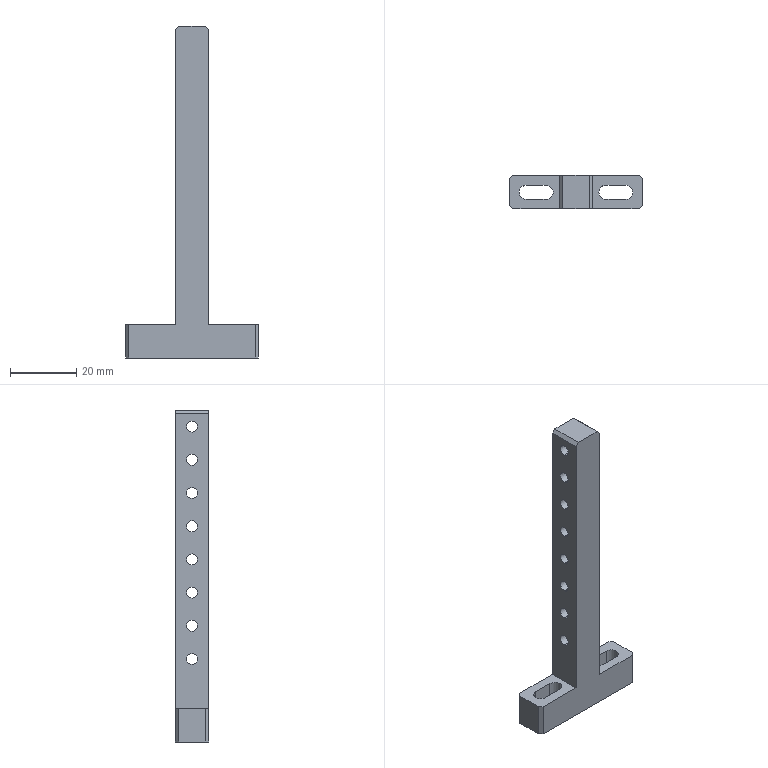Part | SolidWorks | features ICE 3, Chamfer 1, Extrusion 1, HoleWzd 1 | 1 solid | 42 faces | box 40 x 10 x 100 mm | volume 11505 mm3 | cylinder 22 | plane 20 | commonest cylinder face diameters 3.3 x16 4.2 x6
STEP:
#1=CARTESIAN_POINT('',(-5.,0.,26.65));
#2=VERTEX_POINT('',#1);
#3=CARTESIAN_POINT('',(-5.,0.,23.35));
#4=VERTEX_POINT('',#3);
#5=CARTESIAN_POINT('',(-5.,0.,25.));
#6=DIRECTION('',(1.,0.,0.));
#7=DIRECTION('',(0.,0.,-1.));
#8=AXIS2_PLACEMENT_3D('',#5,#6,#7);
#9=CIRCLE('',#8,1.65);
#10=EDGE_CURVE('',#2,#4,#9,.T.);
#11=ORIENTED_EDGE('',*,*,#10,.F.);
#12=CARTESIAN_POINT('',(5.,0.,26.65));
#13=VERTEX_POINT('',#12);
#14=CARTESIAN_POINT('',(5.,0.,26.65));
#15=DIRECTION('',(1.,0.,0.));
#16=VECTOR('',#15,1000.);
#17=LINE('',#14,#16);
#18=EDGE_CURVE('',#2,#13,#17,.T.);
#19=ORIENTED_EDGE('',*,*,#18,.T.);
#20=CARTESIAN_POINT('',(5.,0.,23.35));
#21=VERTEX_POINT('',#20);
#22=CARTESIAN_POINT('',(5.,0.,25.));
#23=DIRECTION('',(1.,0.,0.));
#24=DIRECTION('',(0.,0.,-1.));
#25=AXIS2_PLACEMENT_3D('',#22,#23,#24);
#26=CIRCLE('',#25,1.65);
#27=EDGE_CURVE('',#13,#21,#26,.T.);
#28=ORIENTED_EDGE('',*,*,#27,.T.);
#29=CARTESIAN_POINT('',(5.,0.,23.35));
#30=DIRECTION('',(1.,0.,0.));
#31=VECTOR('',#30,1000.);
#32=LINE('',#29,#31);
#33=EDGE_CURVE('',#4,#21,#32,.T.);
#34=ORIENTED_EDGE('',*,*,#33,.F.);
#35=EDGE_LOOP('',(#11,#19,#28,#34));
#36=FACE_OUTER_BOUND('',#35,.T.);
#37=CARTESIAN_POINT('',(5.,0.,25.));
#38=DIRECTION('',(1.,0.,0.));
#39=DIRECTION('',(0.,0.,-1.));
#40=AXIS2_PLACEMENT_3D('',#37,#38,#39);
#41=CYLINDRICAL_SURFACE('',#40,1.65);
#42=ADVANCED_FACE('',(#36),#41,.F.);
#43=CARTESIAN_POINT('',(-5.,0.,36.65));
#44=VERTEX_POINT('',#43);
#45=CARTESIAN_POINT('',(-5.,0.,33.35));
#46=VERTEX_POINT('',#45);
#47=CARTESIAN_POINT('',(-5.,0.,35.));
#48=DIRECTION('',(1.,0.,0.));
#49=DIRECTION('',(0.,0.,-1.));
#50=AXIS2_PLACEMENT_3D('',#47,#48,#49);
#51=CIRCLE('',#50,1.65);
#52=EDGE_CURVE('',#44,#46,#51,.T.);
#53=ORIENTED_EDGE('',*,*,#52,.F.);
#54=CARTESIAN_POINT('',(5.,0.,36.65));
#55=VERTEX_POINT('',#54);
#56=CARTESIAN_POINT('',(5.,0.,36.65));
#57=DIRECTION('',(1.,0.,0.));
#58=VECTOR('',#57,1000.);
#59=LINE('',#56,#58);
#60=EDGE_CURVE('',#44,#55,#59,.T.);
#61=ORIENTED_EDGE('',*,*,#60,.T.);
#62=CARTESIAN_POINT('',(5.,0.,33.35));
#63=VERTEX_POINT('',#62);
#64=CARTESIAN_POINT('',(5.,0.,35.));
#65=DIRECTION('',(1.,0.,0.));
#66=DIRECTION('',(0.,0.,-1.));
#67=AXIS2_PLACEMENT_3D('',#64,#65,#66);
#68=CIRCLE('',#67,1.65);
#69=EDGE_CURVE('',#55,#63,#68,.T.);
#70=ORIENTED_EDGE('',*,*,#69,.T.);
#71=CARTESIAN_POINT('',(5.,0.,33.35));
#72=DIRECTION('',(1.,0.,0.));
#73=VECTOR('',#72,1000.);
#74=LINE('',#71,#73);
#75=EDGE_CURVE('',#46,#63,#74,.T.);
#76=ORIENTED_EDGE('',*,*,#75,.F.);
#77=EDGE_LOOP('',(#53,#61,#70,#76));
#78=FACE_OUTER_BOUND('',#77,.T.);
#79=CARTESIAN_POINT('',(5.,0.,35.));
#80=DIRECTION('',(1.,0.,0.));
#81=DIRECTION('',(0.,0.,-1.));
#82=AXIS2_PLACEMENT_3D('',#79,#80,#81);
#83=CYLINDRICAL_SURFACE('',#82,1.65);
#84=ADVANCED_FACE('',(#78),#83,.F.);
#85=CARTESIAN_POINT('',(-5.,0.,46.65));
#86=VERTEX_POINT('',#85);
#87=CARTESIAN_POINT('',(-5.,0.,43.35));
#88=VERTEX_POINT('',#87);
#89=CARTESIAN_POINT('',(-5.,0.,45.));
#90=DIRECTION('',(1.,0.,0.));
#91=DIRECTION('',(0.,0.,-1.));
#92=AXIS2_PLACEMENT_3D('',#89,#90,#91);
#93=CIRCLE('',#92,1.65);
#94=EDGE_CURVE('',#86,#88,#93,.T.);
#95=ORIENTED_EDGE('',*,*,#94,.F.);
#96=CARTESIAN_POINT('',(5.,0.,46.65));
#97=VERTEX_POINT('',#96);
#98=CARTESIAN_POINT('',(5.,0.,46.65));
#99=DIRECTION('',(1.,0.,0.));
#100=VECTOR('',#99,1000.);
#101=LINE('',#98,#100);
#102=EDGE_CURVE('',#86,#97,#101,.T.);
#103=ORIENTED_EDGE('',*,*,#102,.T.);
#104=CARTESIAN_POINT('',(5.,0.,43.35));
#105=VERTEX_POINT('',#104);
#106=CARTESIAN_POINT('',(5.,0.,45.));
#107=DIRECTION('',(1.,0.,0.));
#108=DIRECTION('',(0.,0.,-1.));
#109=AXIS2_PLACEMENT_3D('',#106,#107,#108);
#110=CIRCLE('',#109,1.65);
#111=EDGE_CURVE('',#97,#105,#110,.T.);
#112=ORIENTED_EDGE('',*,*,#111,.T.);
#113=CARTESIAN_POINT('',(5.,0.,43.35));
#114=DIRECTION('',(1.,0.,0.));
#115=VECTOR('',#114,1000.);
#116=LINE('',#113,#115);
#117=EDGE_CURVE('',#88,#105,#116,.T.);
#118=ORIENTED_EDGE('',*,*,#117,.F.);
#119=EDGE_LOOP('',(#95,#103,#112,#118));
#120=FACE_OUTER_BOUND('',#119,.T.);
#121=CARTESIAN_POINT('',(5.,0.,45.));
#122=DIRECTION('',(1.,0.,0.));
#123=DIRECTION('',(0.,0.,-1.));
#124=AXIS2_PLACEMENT_3D('',#121,#122,#123);
#125=CYLINDRICAL_SURFACE('',#124,1.65);
#126=ADVANCED_FACE('',(#120),#125,.F.);
#127=CARTESIAN_POINT('',(-5.,0.,56.65));
#128=VERTEX_POINT('',#127);
#129=CARTESIAN_POINT('',(-5.,0.,53.35));
#130=VERTEX_POINT('',#129);
#131=CARTESIAN_POINT('',(-5.,0.,55.));
#132=DIRECTION('',(1.,0.,0.));
#133=DIRECTION('',(0.,0.,-1.));
#134=AXIS2_PLACEMENT_3D('',#131,#132,#133);
#135=CIRCLE('',#134,1.65);
#136=EDGE_CURVE('',#128,#130,#135,.T.);
#137=ORIENTED_EDGE('',*,*,#136,.F.);
#138=CARTESIAN_POINT('',(5.,0.,56.65));
#139=VERTEX_POINT('',#138);
#140=CARTESIAN_POINT('',(5.,0.,56.65));
#141=DIRECTION('',(1.,0.,0.));
#142=VECTOR('',#141,1000.);
#143=LINE('',#140,#142);
#144=EDGE_CURVE('',#128,#139,#143,.T.);
#145=ORIENTED_EDGE('',*,*,#144,.T.);
#146=CARTESIAN_POINT('',(5.,0.,53.35));
#147=VERTEX_POINT('',#146);
#148=CARTESIAN_POINT('',(5.,0.,55.));
#149=DIRECTION('',(1.,0.,0.));
#150=DIRECTION('',(0.,0.,-1.));
#151=AXIS2_PLACEMENT_3D('',#148,#149,#150);
#152=CIRCLE('',#151,1.65);
#153=EDGE_CURVE('',#139,#147,#152,.T.);
#154=ORIENTED_EDGE('',*,*,#153,.T.);
#155=CARTESIAN_POINT('',(5.,0.,53.35));
#156=DIRECTION('',(1.,0.,0.));
#157=VECTOR('',#156,1000.);
#158=LINE('',#155,#157);
#159=EDGE_CURVE('',#130,#147,#158,.T.);
#160=ORIENTED_EDGE('',*,*,#159,.F.);
#161=EDGE_LOOP('',(#137,#145,#154,#160));
#162=FACE_OUTER_BOUND('',#161,.T.);
#163=CARTESIAN_POINT('',(5.,0.,55.));
#164=DIRECTION('',(1.,0.,0.));
#165=DIRECTION('',(0.,0.,-1.));
#166=AXIS2_PLACEMENT_3D('',#163,#164,#165);
#167=CYLINDRICAL_SURFACE('',#166,1.65);
#168=ADVANCED_FACE('',(#162),#167,.F.);
#169=CARTESIAN_POINT('',(-5.,0.,66.65));
#170=VERTEX_POINT('',#169);
#171=CARTESIAN_POINT('',(-5.,0.,63.35));
#172=VERTEX_POINT('',#171);
#173=CARTESIAN_POINT('',(-5.,0.,65.));
#174=DIRECTION('',(1.,0.,0.));
#175=DIRECTION('',(0.,0.,-1.));
#176=AXIS2_PLACEMENT_3D('',#173,#174,#175);
#177=CIRCLE('',#176,1.65);
#178=EDGE_CURVE('',#170,#172,#177,.T.);
#179=ORIENTED_EDGE('',*,*,#178,.F.);
#180=CARTESIAN_POINT('',(5.,0.,66.65));
#181=VERTEX_POINT('',#180);
#182=CARTESIAN_POINT('',(5.,0.,66.65));
#183=DIRECTION('',(1.,0.,0.));
#184=VECTOR('',#183,1000.);
#185=LINE('',#182,#184);
#186=EDGE_CURVE('',#170,#181,#185,.T.);
#187=ORIENTED_EDGE('',*,*,#186,.T.);
#188=CARTESIAN_POINT('',(5.,0.,63.35));
#189=VERTEX_POINT('',#188);
#190=CARTESIAN_POINT('',(5.,0.,65.));
#191=DIRECTION('',(1.,0.,0.));
#192=DIRECTION('',(0.,0.,-1.));
#193=AXIS2_PLACEMENT_3D('',#190,#191,#192);
#194=CIRCLE('',#193,1.65);
#195=EDGE_CURVE('',#181,#189,#194,.T.);
#196=ORIENTED_EDGE('',*,*,#195,.T.);
#197=CARTESIAN_POINT('',(5.,0.,63.35));
#198=DIRECTION('',(1.,0.,0.));
#199=VECTOR('',#198,1000.);
#200=LINE('',#197,#199);
#201=EDGE_CURVE('',#172,#189,#200,.T.);
#202=ORIENTED_EDGE('',*,*,#201,.F.);
#203=EDGE_LOOP('',(#179,#187,#196,#202));
#204=FACE_OUTER_BOUND('',#203,.T.);
#205=CARTESIAN_POINT('',(5.,0.,65.));
#206=DIRECTION('',(1.,0.,0.));
#207=DIRECTION('',(0.,0.,-1.));
#208=AXIS2_PLACEMENT_3D('',#205,#206,#207);
#209=CYLINDRICAL_SURFACE('',#208,1.65);
#210=ADVANCED_FACE('',(#204),#209,.F.);
#211=CARTESIAN_POINT('',(-5.,0.,76.65));
#212=VERTEX_POINT('',#211);
#213=CARTESIAN_POINT('',(-5.,0.,73.35));
#214=VERTEX_POINT('',#213);
#215=CARTESIAN_POINT('',(-5.,0.,75.));
#216=DIRECTION('',(1.,0.,0.));
#217=DIRECTION('',(0.,0.,-1.));
#218=AXIS2_PLACEMENT_3D('',#215,#216,#217);
#219=CIRCLE('',#218,1.65);
#220=EDGE_CURVE('',#212,#214,#219,.T.);
#221=ORIENTED_EDGE('',*,*,#220,.F.);
#222=CARTESIAN_POINT('',(5.,0.,76.65));
#223=VERTEX_POINT('',#222);
#224=CARTESIAN_POINT('',(5.,0.,76.65));
#225=DIRECTION('',(1.,0.,0.));
#226=VECTOR('',#225,1000.);
#227=LINE('',#224,#226);
#228=EDGE_CURVE('',#212,#223,#227,.T.);
#229=ORIENTED_EDGE('',*,*,#228,.T.);
#230=CARTESIAN_POINT('',(5.,0.,73.35));
#231=VERTEX_POINT('',#230);
#232=CARTESIAN_POINT('',(5.,0.,75.));
#233=DIRECTION('',(1.,0.,0.));
#234=DIRECTION('',(0.,0.,-1.));
#235=AXIS2_PLACEMENT_3D('',#232,#233,#234);
#236=CIRCLE('',#235,1.65);
#237=EDGE_CURVE('',#223,#231,#236,.T.);
#238=ORIENTED_EDGE('',*,*,#237,.T.);
#239=CARTESIAN_POINT('',(5.,0.,73.35));
#240=DIRECTION('',(1.,0.,0.));
#241=VECTOR('',#240,1000.);
#242=LINE('',#239,#241);
#243=EDGE_CURVE('',#214,#231,#242,.T.);
#244=ORIENTED_EDGE('',*,*,#243,.F.);
#245=EDGE_LOOP('',(#221,#229,#238,#244));
#246=FACE_OUTER_BOUND('',#245,.T.);
#247=CARTESIAN_POINT('',(5.,0.,75.));
#248=DIRECTION('',(1.,0.,0.));
#249=DIRECTION('',(0.,0.,-1.));
#250=AXIS2_PLACEMENT_3D('',#247,#248,#249);
#251=CYLINDRICAL_SURFACE('',#250,1.65);
#252=ADVANCED_FACE('',(#246),#251,.F.);
#253=CARTESIAN_POINT('',(-5.,0.,86.65));
#254=VERTEX_POINT('',#253);
#255=CARTESIAN_POINT('',(-5.,0.,83.35));
#256=VERTEX_POINT('',#255);
#257=CARTESIAN_POINT('',(-5.,0.,85.));
#258=DIRECTION('',(1.,0.,0.));
#259=DIRECTION('',(0.,0.,-1.));
#260=AXIS2_PLACEMENT_3D('',#257,#258,#259);
#261=CIRCLE('',#260,1.65);
#262=EDGE_CURVE('',#254,#256,#261,.T.);
#263=ORIENTED_EDGE('',*,*,#262,.F.);
#264=CARTESIAN_POINT('',(5.,0.,86.65));
#265=VERTEX_POINT('',#264);
#266=CARTESIAN_POINT('',(5.,0.,86.65));
#267=DIRECTION('',(1.,0.,0.));
#268=VECTOR('',#267,1000.);
#269=LINE('',#266,#268);
#270=EDGE_CURVE('',#254,#265,#269,.T.);
#271=ORIENTED_EDGE('',*,*,#270,.T.);
#272=CARTESIAN_POINT('',(5.,0.,83.35));
#273=VERTEX_POINT('',#272);
#274=CARTESIAN_POINT('',(5.,0.,85.));
#275=DIRECTION('',(1.,0.,0.));
#276=DIRECTION('',(0.,0.,-1.));
#277=AXIS2_PLACEMENT_3D('',#274,#275,#276);
#278=CIRCLE('',#277,1.65);
#279=EDGE_CURVE('',#265,#273,#278,.T.);
#280=ORIENTED_EDGE('',*,*,#279,.T.);
#281=CARTESIAN_POINT('',(5.,0.,83.35));
#282=DIRECTION('',(1.,0.,0.));
#283=VECTOR('',#282,1000.);
#284=LINE('',#281,#283);
#285=EDGE_CURVE('',#256,#273,#284,.T.);
#286=ORIENTED_EDGE('',*,*,#285,.F.);
#287=EDGE_LOOP('',(#263,#271,#280,#286));
#288=FACE_OUTER_BOUND('',#287,.T.);
#289=CARTESIAN_POINT('',(5.,0.,85.));
#290=DIRECTION('',(1.,0.,0.));
#291=DIRECTION('',(0.,0.,-1.));
#292=AXIS2_PLACEMENT_3D('',#289,#290,#291);
#293=CYLINDRICAL_SURFACE('',#292,1.65);
#294=ADVANCED_FACE('',(#288),#293,.F.);
#295=CARTESIAN_POINT('',(-5.,0.,96.65));
#296=VERTEX_POINT('',#295);
#297=CARTESIAN_POINT('',(-5.,0.,93.35));
#298=VERTEX_POINT('',#297);
#299=CARTESIAN_POINT('',(-5.,0.,95.));
#300=DIRECTION('',(1.,0.,0.));
#301=DIRECTION('',(0.,0.,-1.));
#302=AXIS2_PLACEMENT_3D('',#299,#300,#301);
#303=CIRCLE('',#302,1.65);
#304=EDGE_CURVE('',#296,#298,#303,.T.);
#305=ORIENTED_EDGE('',*,*,#304,.F.);
#306=CARTESIAN_POINT('',(5.,0.,96.65));
#307=VERTEX_POINT('',#306);
#308=CARTESIAN_POINT('',(5.,0.,96.65));
#309=DIRECTION('',(1.,0.,0.));
#310=VECTOR('',#309,1000.);
#311=LINE('',#308,#310);
#312=EDGE_CURVE('',#296,#307,#311,.T.);
#313=ORIENTED_EDGE('',*,*,#312,.T.);
#314=CARTESIAN_POINT('',(5.,0.,93.35));
#315=VERTEX_POINT('',#314);
#316=CARTESIAN_POINT('',(5.,0.,95.));
#317=DIRECTION('',(1.,0.,0.));
#318=DIRECTION('',(0.,0.,-1.));
#319=AXIS2_PLACEMENT_3D('',#316,#317,#318);
#320=CIRCLE('',#319,1.65);
#321=EDGE_CURVE('',#307,#315,#320,.T.);
#322=ORIENTED_EDGE('',*,*,#321,.T.);
#323=CARTESIAN_POINT('',(5.,0.,93.35));
#324=DIRECTION('',(1.,0.,0.));
#325=VECTOR('',#324,1000.);
#326=LINE('',#323,#325);
#327=EDGE_CURVE('',#298,#315,#326,.T.);
#328=ORIENTED_EDGE('',*,*,#327,.F.);
#329=EDGE_LOOP('',(#305,#313,#322,#328));
#330=FACE_OUTER_BOUND('',#329,.T.);
#331=CARTESIAN_POINT('',(5.,0.,95.));
#332=DIRECTION('',(1.,0.,0.));
#333=DIRECTION('',(0.,0.,-1.));
#334=AXIS2_PLACEMENT_3D('',#331,#332,#333);
#335=CYLINDRICAL_SURFACE('',#334,1.65);
#336=ADVANCED_FACE('',(#330),#335,.F.);
#337=CARTESIAN_POINT('',(-15.,2.1,10.));
#338=VERTEX_POINT('',#337);
#339=CARTESIAN_POINT('',(-17.1,0.,10.));
#340=VERTEX_POINT('',#339);
#341=CARTESIAN_POINT('',(-15.,0.,10.));
#342=DIRECTION('',(0.,0.,1.));
#343=DIRECTION('',(1.,0.,0.));
#344=AXIS2_PLACEMENT_3D('',#341,#342,#343);
#345=CIRCLE('',#344,2.1);
#346=EDGE_CURVE('',#338,#340,#345,.T.);
#347=ORIENTED_EDGE('',*,*,#346,.T.);
#348=CARTESIAN_POINT('',(-17.1,0.,0.));
#349=VERTEX_POINT('',#348);
#350=CARTESIAN_POINT('',(-17.1,0.,100.));
#351=DIRECTION('',(0.,0.,-1.));
#352=VECTOR('',#351,1000.);
#353=LINE('',#350,#352);
#354=EDGE_CURVE('',#340,#349,#353,.T.);
#355=ORIENTED_EDGE('',*,*,#354,.T.);
#356=CARTESIAN_POINT('',(-15.,2.1,0.));
#357=VERTEX_POINT('',#356);
#358=CARTESIAN_POINT('',(-15.,0.,0.));
#359=DIRECTION('',(0.,0.,-1.));
#360=DIRECTION('',(1.,0.,0.));
#361=AXIS2_PLACEMENT_3D('',#358,#359,#360);
#362=CIRCLE('',#361,2.1);
#363=EDGE_CURVE('',#349,#357,#362,.T.);
#364=ORIENTED_EDGE('',*,*,#363,.T.);
#365=CARTESIAN_POINT('',(-15.,2.1,100.));
#366=DIRECTION('',(0.,0.,-1.));
#367=VECTOR('',#366,1000.);
#368=LINE('',#365,#367);
#369=EDGE_CURVE('',#338,#357,#368,.T.);
#370=ORIENTED_EDGE('',*,*,#369,.F.);
#371=EDGE_LOOP('',(#347,#355,#364,#370));
#372=FACE_OUTER_BOUND('',#371,.T.);
#373=CARTESIAN_POINT('',(-15.,0.,100.));
#374=DIRECTION('',(0.,0.,-1.));
#375=DIRECTION('',(-1.,0.,0.));
#376=AXIS2_PLACEMENT_3D('',#373,#374,#375);
#377=CYLINDRICAL_SURFACE('',#376,2.1);
#378=ADVANCED_FACE('',(#372),#377,.F.);
#379=CARTESIAN_POINT('',(9.,2.1,10.));
#380=VERTEX_POINT('',#379);
#381=CARTESIAN_POINT('',(6.9,0.,10.));
#382=VERTEX_POINT('',#381);
#383=CARTESIAN_POINT('',(9.,0.,10.));
#384=DIRECTION('',(0.,0.,1.));
#385=DIRECTION('',(1.,0.,0.));
#386=AXIS2_PLACEMENT_3D('',#383,#384,#385);
#387=CIRCLE('',#386,2.1);
#388=EDGE_CURVE('',#380,#382,#387,.T.);
#389=ORIENTED_EDGE('',*,*,#388,.T.);
#390=CARTESIAN_POINT('',(6.9,0.,0.));
#391=VERTEX_POINT('',#390);
#392=CARTESIAN_POINT('',(6.9,0.,100.));
#393=DIRECTION('',(0.,0.,-1.));
#394=VECTOR('',#393,1000.);
#395=LINE('',#392,#394);
#396=EDGE_CURVE('',#382,#391,#395,.T.);
#397=ORIENTED_EDGE('',*,*,#396,.T.);
#398=CARTESIAN_POINT('',(9.,2.1,0.));
#399=VERTEX_POINT('',#398);
#400=CARTESIAN_POINT('',(9.,0.,0.));
#401=DIRECTION('',(0.,0.,-1.));
#402=DIRECTION('',(-1.,0.,0.));
#403=AXIS2_PLACEMENT_3D('',#400,#401,#402);
#404=CIRCLE('',#403,2.1);
#405=EDGE_CURVE('',#391,#399,#404,.T.);
#406=ORIENTED_EDGE('',*,*,#405,.T.);
#407=CARTESIAN_POINT('',(9.,2.1,100.));
#408=DIRECTION('',(0.,0.,-1.));
#409=VECTOR('',#408,1000.);
#410=LINE('',#407,#409);
#411=EDGE_CURVE('',#380,#399,#410,.T.);
#412=ORIENTED_EDGE('',*,*,#411,.F.);
#413=EDGE_LOOP('',(#389,#397,#406,#412));
#414=FACE_OUTER_BOUND('',#413,.T.);
#415=CARTESIAN_POINT('',(9.,0.,100.));
#416=DIRECTION('',(0.,0.,-1.));
#417=DIRECTION('',(-1.,0.,0.));
#418=AXIS2_PLACEMENT_3D('',#415,#416,#417);
#419=CYLINDRICAL_SURFACE('',#418,2.1);
#420=ADVANCED_FACE('',(#414),#419,.F.);
#421=CARTESIAN_POINT('',(15.,-2.1,10.));
#422=VERTEX_POINT('',#421);
#423=CARTESIAN_POINT('',(15.,2.1,10.));
#424=VERTEX_POINT('',#423);
#425=CARTESIAN_POINT('',(15.,0.,10.));
#426=DIRECTION('',(0.,0.,1.));
#427=DIRECTION('',(1.,0.,0.));
#428=AXIS2_PLACEMENT_3D('',#425,#426,#427);
#429=CIRCLE('',#428,2.1);
#430=EDGE_CURVE('',#422,#424,#429,.T.);
#431=ORIENTED_EDGE('',*,*,#430,.F.);
#432=CARTESIAN_POINT('',(9.,-2.1,10.));
#433=VERTEX_POINT('',#432);
#434=CARTESIAN_POINT('',(20.,-2.1,10.));
#435=DIRECTION('',(1.,0.,0.));
#436=VECTOR('',#435,1000.);
#437=LINE('',#434,#436);
#438=EDGE_CURVE('',#433,#422,#437,.T.);
#439=ORIENTED_EDGE('',*,*,#438,.F.);
#440=CARTESIAN_POINT('',(9.,0.,10.));
#441=DIRECTION('',(0.,0.,1.));
#442=DIRECTION('',(1.,0.,0.));
#443=AXIS2_PLACEMENT_3D('',#440,#441,#442);
#444=CIRCLE('',#443,2.1);
#445=EDGE_CURVE('',#382,#433,#444,.T.);
#446=ORIENTED_EDGE('',*,*,#445,.F.);
#447=ORIENTED_EDGE('',*,*,#388,.F.);
#448=CARTESIAN_POINT('',(20.,2.1,10.));
#449=DIRECTION('',(-1.,0.,0.));
#450=VECTOR('',#449,1000.);
#451=LINE('',#448,#450);
#452=EDGE_CURVE('',#424,#380,#451,.T.);
#453=ORIENTED_EDGE('',*,*,#452,.F.);
#454=EDGE_LOOP('',(#431,#439,#446,#447,#453));
#455=FACE_BOUND('',#454,.T.);
#456=CARTESIAN_POINT('',(20.,-4.,10.));
#457=VERTEX_POINT('',#456);
#458=CARTESIAN_POINT('',(20.,4.,10.));
#459=VERTEX_POINT('',#458);
#460=CARTESIAN_POINT('',(20.,5.,10.));
#461=DIRECTION('',(0.,1.,0.));
#462=VECTOR('',#461,1000.);
#463=LINE('',#460,#462);
#464=EDGE_CURVE('',#457,#459,#463,.T.);
#465=ORIENTED_EDGE('',*,*,#464,.T.);
#466=CARTESIAN_POINT('',(19.,5.,10.));
#467=VERTEX_POINT('',#466);
#468=CARTESIAN_POINT('',(24.5,-0.5,10.));
#469=DIRECTION('',(-0.7071,0.7071,0.));
#470=VECTOR('',#469,1000.);
#471=LINE('',#468,#470);
#472=EDGE_CURVE('',#459,#467,#471,.T.);
#473=ORIENTED_EDGE('',*,*,#472,.T.);
#474=CARTESIAN_POINT('',(5.,5.,10.));
#475=VERTEX_POINT('',#474);
#476=CARTESIAN_POINT('',(-20.,5.,10.));
#477=DIRECTION('',(-1.,0.,0.));
#478=VECTOR('',#477,1000.);
#479=LINE('',#476,#478);
#480=EDGE_CURVE('',#467,#475,#479,.T.);
#481=ORIENTED_EDGE('',*,*,#480,.T.);
#482=CARTESIAN_POINT('',(5.,-5.,10.));
#483=VERTEX_POINT('',#482);
#484=CARTESIAN_POINT('',(5.,-5.,10.));
#485=DIRECTION('',(0.,1.,0.));
#486=VECTOR('',#485,1000.);
#487=LINE('',#484,#486);
#488=EDGE_CURVE('',#483,#475,#487,.T.);
#489=ORIENTED_EDGE('',*,*,#488,.F.);
#490=CARTESIAN_POINT('',(19.,-5.,10.));
#491=VERTEX_POINT('',#490);
#492=CARTESIAN_POINT('',(-20.,-5.,10.));
#493=DIRECTION('',(1.,0.,0.));
#494=VECTOR('',#493,1000.);
#495=LINE('',#492,#494);
#496=EDGE_CURVE('',#483,#491,#495,.T.);
#497=ORIENTED_EDGE('',*,*,#496,.T.);
#498=CARTESIAN_POINT('',(19.5,-4.5,10.));
#499=DIRECTION('',(0.7071,0.7071,0.));
#500=VECTOR('',#499,1000.);
#501=LINE('',#498,#500);
#502=EDGE_CURVE('',#491,#457,#501,.T.);
#503=ORIENTED_EDGE('',*,*,#502,.T.);
#504=EDGE_LOOP('',(#465,#473,#481,#489,#497,#503));
#505=FACE_OUTER_BOUND('',#504,.T.);
#506=CARTESIAN_POINT('',(20.,-5.,10.));
#507=DIRECTION('',(0.,0.,1.));
#508=DIRECTION('',(1.,0.,0.));
#509=AXIS2_PLACEMENT_3D('',#506,#507,#508);
#510=PLANE('',#509);
#511=ADVANCED_FACE('',(#455,#505),#510,.T.);
#512=CARTESIAN_POINT('',(20.,-4.,0.));
#513=VERTEX_POINT('',#512);
#514=CARTESIAN_POINT('',(20.,4.,0.));
#515=VERTEX_POINT('',#514);
#516=CARTESIAN_POINT('',(20.,5.,0.));
#517=DIRECTION('',(0.,1.,0.));
#518=VECTOR('',#517,1000.);
#519=LINE('',#516,#518);
#520=EDGE_CURVE('',#513,#515,#519,.T.);
#521=ORIENTED_EDGE('',*,*,#520,.T.);
#522=CARTESIAN_POINT('',(20.,4.,10.));
#523=DIRECTION('',(0.,0.,1.));
#524=VECTOR('',#523,1000.);
#525=LINE('',#522,#524);
#526=EDGE_CURVE('',#515,#459,#525,.T.);
#527=ORIENTED_EDGE('',*,*,#526,.T.);
#528=ORIENTED_EDGE('',*,*,#464,.F.);
#529=CARTESIAN_POINT('',(20.,-4.,10.));
#530=DIRECTION('',(0.,0.,-1.));
#531=VECTOR('',#530,1000.);
#532=LINE('',#529,#531);
#533=EDGE_CURVE('',#457,#513,#532,.T.);
#534=ORIENTED_EDGE('',*,*,#533,.T.);
#535=EDGE_LOOP('',(#521,#527,#528,#534));
#536=FACE_OUTER_BOUND('',#535,.T.);
#537=CARTESIAN_POINT('',(20.,5.,10.));
#538=DIRECTION('',(-1.,0.,0.));
#539=DIRECTION('',(0.,-1.,0.));
#540=AXIS2_PLACEMENT_3D('',#537,#538,#539);
#541=PLANE('',#540);
#542=ADVANCED_FACE('',(#536),#541,.F.);
#543=ORIENTED_EDGE('',*,*,#480,.F.);
#544=CARTESIAN_POINT('',(19.,5.,0.));
#545=VERTEX_POINT('',#544);
#546=CARTESIAN_POINT('',(19.,5.,10.));
#547=DIRECTION('',(0.,0.,-1.));
#548=VECTOR('',#547,1000.);
#549=LINE('',#546,#548);
#550=EDGE_CURVE('',#467,#545,#549,.T.);
#551=ORIENTED_EDGE('',*,*,#550,.T.);
#552=CARTESIAN_POINT('',(-19.,5.,0.));
#553=VERTEX_POINT('',#552);
#554=CARTESIAN_POINT('',(-20.,5.,0.));
#555=DIRECTION('',(-1.,0.,0.));
#556=VECTOR('',#555,1000.);
#557=LINE('',#554,#556);
#558=EDGE_CURVE('',#545,#553,#557,.T.);
#559=ORIENTED_EDGE('',*,*,#558,.T.);
#560=CARTESIAN_POINT('',(-19.,5.,10.));
#561=VERTEX_POINT('',#560);
#562=CARTESIAN_POINT('',(-19.,5.,10.));
#563=DIRECTION('',(0.,0.,1.));
#564=VECTOR('',#563,1000.);
#565=LINE('',#562,#564);
#566=EDGE_CURVE('',#553,#561,#565,.T.);
#567=ORIENTED_EDGE('',*,*,#566,.T.);
#568=CARTESIAN_POINT('',(-5.,5.,10.));
#569=VERTEX_POINT('',#568);
#570=CARTESIAN_POINT('',(-20.,5.,10.));
#571=DIRECTION('',(-1.,0.,0.));
#572=VECTOR('',#571,1000.);
#573=LINE('',#570,#572);
#574=EDGE_CURVE('',#569,#561,#573,.T.);
#575=ORIENTED_EDGE('',*,*,#574,.F.);
#576=CARTESIAN_POINT('',(-5.,5.,99.));
#577=VERTEX_POINT('',#576);
#578=CARTESIAN_POINT('',(-5.,5.,100.));
#579=DIRECTION('',(0.,0.,-1.));
#580=VECTOR('',#579,1000.);
#581=LINE('',#578,#580);
#582=EDGE_CURVE('',#577,#569,#581,.T.);
#583=ORIENTED_EDGE('',*,*,#582,.F.);
#584=CARTESIAN_POINT('',(-4.,5.,100.));
#585=VERTEX_POINT('',#584);
#586=CARTESIAN_POINT('',(-4.,5.,100.));
#587=DIRECTION('',(0.7071,0.,0.7071));
#588=VECTOR('',#587,1000.);
#589=LINE('',#586,#588);
#590=EDGE_CURVE('',#577,#585,#589,.T.);
#591=ORIENTED_EDGE('',*,*,#590,.T.);
#592=CARTESIAN_POINT('',(4.,5.,100.));
#593=VERTEX_POINT('',#592);
#594=CARTESIAN_POINT('',(-5.,5.,100.));
#595=DIRECTION('',(-1.,0.,0.));
#596=VECTOR('',#595,1000.);
#597=LINE('',#594,#596);
#598=EDGE_CURVE('',#593,#585,#597,.T.);
#599=ORIENTED_EDGE('',*,*,#598,.F.);
#600=CARTESIAN_POINT('',(5.,5.,99.));
#601=VERTEX_POINT('',#600);
#602=CARTESIAN_POINT('',(4.,5.,100.));
#603=DIRECTION('',(0.7071,0.,-0.7071));
#604=VECTOR('',#603,1000.);
#605=LINE('',#602,#604);
#606=EDGE_CURVE('',#593,#601,#605,.T.);
#607=ORIENTED_EDGE('',*,*,#606,.T.);
#608=CARTESIAN_POINT('',(5.,5.,100.));
#609=DIRECTION('',(0.,0.,-1.));
#610=VECTOR('',#609,1000.);
#611=LINE('',#608,#610);
#612=EDGE_CURVE('',#601,#475,#611,.T.);
#613=ORIENTED_EDGE('',*,*,#612,.T.);
#614=EDGE_LOOP('',(#543,#551,#559,#567,#575,#583,#591,#599,#607,#613));
#615=FACE_OUTER_BOUND('',#614,.T.);
#616=CARTESIAN_POINT('',(-20.,5.,10.));
#617=DIRECTION('',(0.,-1.,0.));
#618=DIRECTION('',(0.,0.,-1.));
#619=AXIS2_PLACEMENT_3D('',#616,#617,#618);
#620=PLANE('',#619);
#621=ADVANCED_FACE('',(#615),#620,.F.);
#622=CARTESIAN_POINT('',(-20.,4.,0.));
#623=VERTEX_POINT('',#622);
#624=CARTESIAN_POINT('',(-20.,-4.,0.));
#625=VERTEX_POINT('',#624);
#626=CARTESIAN_POINT('',(-20.,5.,0.));
#627=DIRECTION('',(0.,-1.,0.));
#628=VECTOR('',#627,1000.);
#629=LINE('',#626,#628);
#630=EDGE_CURVE('',#623,#625,#629,.T.);
#631=ORIENTED_EDGE('',*,*,#630,.T.);
#632=CARTESIAN_POINT('',(-20.,-4.,10.));
#633=VERTEX_POINT('',#632);
#634=CARTESIAN_POINT('',(-20.,-4.,10.));
#635=DIRECTION('',(0.,0.,1.));
#636=VECTOR('',#635,1000.);
#637=LINE('',#634,#636);
#638=EDGE_CURVE('',#625,#633,#637,.T.);
#639=ORIENTED_EDGE('',*,*,#638,.T.);
#640=CARTESIAN_POINT('',(-20.,4.,10.));
#641=VERTEX_POINT('',#640);
#642=CARTESIAN_POINT('',(-20.,5.,10.));
#643=DIRECTION('',(0.,-1.,0.));
#644=VECTOR('',#643,1000.);
#645=LINE('',#642,#644);
#646=EDGE_CURVE('',#641,#633,#645,.T.);
#647=ORIENTED_EDGE('',*,*,#646,.F.);
#648=CARTESIAN_POINT('',(-20.,4.,10.));
#649=DIRECTION('',(0.,0.,-1.));
#650=VECTOR('',#649,1000.);
#651=LINE('',#648,#650);
#652=EDGE_CURVE('',#641,#623,#651,.T.);
#653=ORIENTED_EDGE('',*,*,#652,.T.);
#654=EDGE_LOOP('',(#631,#639,#647,#653));
#655=FACE_OUTER_BOUND('',#654,.T.);
#656=CARTESIAN_POINT('',(-20.,5.,10.));
#657=DIRECTION('',(1.,0.,0.));
#658=DIRECTION('',(0.,0.,-1.));
#659=AXIS2_PLACEMENT_3D('',#656,#657,#658);
#660=PLANE('',#659);
#661=ADVANCED_FACE('',(#655),#660,.F.);
#662=CARTESIAN_POINT('',(-19.,-5.,0.));
#663=VERTEX_POINT('',#662);
#664=CARTESIAN_POINT('',(19.,-5.,0.));
#665=VERTEX_POINT('',#664);
#666=CARTESIAN_POINT('',(-20.,-5.,0.));
#667=DIRECTION('',(1.,0.,0.));
#668=VECTOR('',#667,1000.);
#669=LINE('',#666,#668);
#670=EDGE_CURVE('',#663,#665,#669,.T.);
#671=ORIENTED_EDGE('',*,*,#670,.T.);
#672=CARTESIAN_POINT('',(19.,-5.,10.));
#673=DIRECTION('',(0.,0.,1.));
#674=VECTOR('',#673,1000.);
#675=LINE('',#672,#674);
#676=EDGE_CURVE('',#665,#491,#675,.T.);
#677=ORIENTED_EDGE('',*,*,#676,.T.);
#678=ORIENTED_EDGE('',*,*,#496,.F.);
#679=CARTESIAN_POINT('',(5.,-5.,99.));
#680=VERTEX_POINT('',#679);
#681=CARTESIAN_POINT('',(5.,-5.,100.));
#682=DIRECTION('',(0.,0.,-1.));
#683=VECTOR('',#682,1000.);
#684=LINE('',#681,#683);
#685=EDGE_CURVE('',#680,#483,#684,.T.);
#686=ORIENTED_EDGE('',*,*,#685,.F.);
#687=CARTESIAN_POINT('',(4.,-5.,100.));
#688=VERTEX_POINT('',#687);
#689=CARTESIAN_POINT('',(4.,-5.,100.));
#690=DIRECTION('',(-0.7071,0.,0.7071));
#691=VECTOR('',#690,1000.);
#692=LINE('',#689,#691);
#693=EDGE_CURVE('',#680,#688,#692,.T.);
#694=ORIENTED_EDGE('',*,*,#693,.T.);
#695=CARTESIAN_POINT('',(-4.,-5.,100.));
#696=VERTEX_POINT('',#695);
#697=CARTESIAN_POINT('',(-5.,-5.,100.));
#698=DIRECTION('',(1.,0.,0.));
#699=VECTOR('',#698,1000.);
#700=LINE('',#697,#699);
#701=EDGE_CURVE('',#696,#688,#700,.T.);
#702=ORIENTED_EDGE('',*,*,#701,.F.);
#703=CARTESIAN_POINT('',(-5.,-5.,99.));
#704=VERTEX_POINT('',#703);
#705=CARTESIAN_POINT('',(-4.,-5.,100.));
#706=DIRECTION('',(-0.7071,0.,-0.7071));
#707=VECTOR('',#706,1000.);
#708=LINE('',#705,#707);
#709=EDGE_CURVE('',#696,#704,#708,.T.);
#710=ORIENTED_EDGE('',*,*,#709,.T.);
#711=CARTESIAN_POINT('',(-5.,-5.,10.));
#712=VERTEX_POINT('',#711);
#713=CARTESIAN_POINT('',(-5.,-5.,100.));
#714=DIRECTION('',(0.,0.,-1.));
#715=VECTOR('',#714,1000.);
#716=LINE('',#713,#715);
#717=EDGE_CURVE('',#704,#712,#716,.T.);
#718=ORIENTED_EDGE('',*,*,#717,.T.);
#719=CARTESIAN_POINT('',(-19.,-5.,10.));
#720=VERTEX_POINT('',#719);
#721=CARTESIAN_POINT('',(-20.,-5.,10.));
#722=DIRECTION('',(1.,0.,0.));
#723=VECTOR('',#722,1000.);
#724=LINE('',#721,#723);
#725=EDGE_CURVE('',#720,#712,#724,.T.);
#726=ORIENTED_EDGE('',*,*,#725,.F.);
#727=CARTESIAN_POINT('',(-19.,-5.,10.));
#728=DIRECTION('',(0.,0.,-1.));
#729=VECTOR('',#728,1000.);
#730=LINE('',#727,#729);
#731=EDGE_CURVE('',#720,#663,#730,.T.);
#732=ORIENTED_EDGE('',*,*,#731,.T.);
#733=EDGE_LOOP('',(#671,#677,#678,#686,#694,#702,#710,#718,#726,#732));
#734=FACE_OUTER_BOUND('',#733,.T.);
#735=CARTESIAN_POINT('',(-20.,-5.,10.));
#736=DIRECTION('',(0.,1.,0.));
#737=DIRECTION('',(0.,0.,1.));
#738=AXIS2_PLACEMENT_3D('',#735,#736,#737);
#739=PLANE('',#738);
#740=ADVANCED_FACE('',(#734),#739,.F.);
#741=ORIENTED_EDGE('',*,*,#346,.F.);
#742=CARTESIAN_POINT('',(-9.,2.1,10.));
#743=VERTEX_POINT('',#742);
#744=CARTESIAN_POINT('',(20.,2.1,10.));
#745=DIRECTION('',(-1.,0.,0.));
#746=VECTOR('',#745,1000.);
#747=LINE('',#744,#746);
#748=EDGE_CURVE('',#743,#338,#747,.T.);
#749=ORIENTED_EDGE('',*,*,#748,.F.);
#750=CARTESIAN_POINT('',(-9.,-2.1,10.));
#751=VERTEX_POINT('',#750);
#752=CARTESIAN_POINT('',(-9.,0.,10.));
#753=DIRECTION('',(0.,0.,1.));
#754=DIRECTION('',(1.,0.,0.));
#755=AXIS2_PLACEMENT_3D('',#752,#753,#754);
#756=CIRCLE('',#755,2.1);
#757=EDGE_CURVE('',#751,#743,#756,.T.);
#758=ORIENTED_EDGE('',*,*,#757,.F.);
#759=CARTESIAN_POINT('',(-15.,-2.1,10.));
#760=VERTEX_POINT('',#759);
#761=CARTESIAN_POINT('',(20.,-2.1,10.));
#762=DIRECTION('',(1.,0.,0.));
#763=VECTOR('',#762,1000.);
#764=LINE('',#761,#763);
#765=EDGE_CURVE('',#760,#751,#764,.T.);
#766=ORIENTED_EDGE('',*,*,#765,.F.);
#767=CARTESIAN_POINT('',(-15.,0.,10.));
#768=DIRECTION('',(0.,0.,1.));
#769=DIRECTION('',(1.,0.,0.));
#770=AXIS2_PLACEMENT_3D('',#767,#768,#769);
#771=CIRCLE('',#770,2.1);
#772=EDGE_CURVE('',#340,#760,#771,.T.);
#773=ORIENTED_EDGE('',*,*,#772,.F.);
#774=EDGE_LOOP('',(#741,#749,#758,#766,#773));
#775=FACE_BOUND('',#774,.T.);
#776=ORIENTED_EDGE('',*,*,#646,.T.);
#777=CARTESIAN_POINT('',(0.5,-24.5,10.));
#778=DIRECTION('',(0.7071,-0.7071,0.));
#779=VECTOR('',#778,1000.);
#780=LINE('',#777,#779);
#781=EDGE_CURVE('',#633,#720,#780,.T.);
#782=ORIENTED_EDGE('',*,*,#781,.T.);
#783=ORIENTED_EDGE('',*,*,#725,.T.);
#784=CARTESIAN_POINT('',(-5.,-5.,10.));
#785=DIRECTION('',(0.,-1.,0.));
#786=VECTOR('',#785,1000.);
#787=LINE('',#784,#786);
#788=EDGE_CURVE('',#569,#712,#787,.T.);
#789=ORIENTED_EDGE('',*,*,#788,.F.);
#790=ORIENTED_EDGE('',*,*,#574,.T.);
#791=CARTESIAN_POINT('',(-4.5,19.5,10.));
#792=DIRECTION('',(-0.7071,-0.7071,0.));
#793=VECTOR('',#792,1000.);
#794=LINE('',#791,#793);
#795=EDGE_CURVE('',#561,#641,#794,.T.);
#796=ORIENTED_EDGE('',*,*,#795,.T.);
#797=EDGE_LOOP('',(#776,#782,#783,#789,#790,#796));
#798=FACE_OUTER_BOUND('',#797,.T.);
#799=CARTESIAN_POINT('',(20.,-5.,10.));
#800=DIRECTION('',(0.,0.,1.));
#801=DIRECTION('',(1.,0.,0.));
#802=AXIS2_PLACEMENT_3D('',#799,#800,#801);
#803=PLANE('',#802);
#804=ADVANCED_FACE('',(#775,#798),#803,.T.);
#805=CARTESIAN_POINT('',(-9.,2.1,0.));
#806=VERTEX_POINT('',#805);
#807=CARTESIAN_POINT('',(-15.,2.1,0.));
#808=DIRECTION('',(1.,0.,0.));
#809=VECTOR('',#808,1000.);
#810=LINE('',#807,#809);
#811=EDGE_CURVE('',#357,#806,#810,.T.);
#812=ORIENTED_EDGE('',*,*,#811,.F.);
#813=ORIENTED_EDGE('',*,*,#363,.F.);
#814=CARTESIAN_POINT('',(-15.,-2.1,0.));
#815=VERTEX_POINT('',#814);
#816=CARTESIAN_POINT('',(-15.,0.,0.));
#817=DIRECTION('',(0.,0.,-1.));
#818=DIRECTION('',(1.,0.,0.));
#819=AXIS2_PLACEMENT_3D('',#816,#817,#818);
#820=CIRCLE('',#819,2.1);
#821=EDGE_CURVE('',#815,#349,#820,.T.);
#822=ORIENTED_EDGE('',*,*,#821,.F.);
#823=CARTESIAN_POINT('',(-9.,-2.1,0.));
#824=VERTEX_POINT('',#823);
#825=CARTESIAN_POINT('',(-15.,-2.1,0.));
#826=DIRECTION('',(-1.,0.,0.));
#827=VECTOR('',#826,1000.);
#828=LINE('',#825,#827);
#829=EDGE_CURVE('',#824,#815,#828,.T.);
#830=ORIENTED_EDGE('',*,*,#829,.F.);
#831=CARTESIAN_POINT('',(-9.,0.,0.));
#832=DIRECTION('',(0.,0.,-1.));
#833=DIRECTION('',(1.,0.,0.));
#834=AXIS2_PLACEMENT_3D('',#831,#832,#833);
#835=CIRCLE('',#834,2.1);
#836=EDGE_CURVE('',#806,#824,#835,.T.);
#837=ORIENTED_EDGE('',*,*,#836,.F.);
#838=EDGE_LOOP('',(#812,#813,#822,#830,#837));
#839=FACE_BOUND('',#838,.T.);
#840=CARTESIAN_POINT('',(15.,-2.1,0.));
#841=VERTEX_POINT('',#840);
#842=CARTESIAN_POINT('',(9.,-2.1,0.));
#843=VERTEX_POINT('',#842);
#844=CARTESIAN_POINT('',(15.,-2.1,0.));
#845=DIRECTION('',(-1.,0.,0.));
#846=VECTOR('',#845,1000.);
#847=LINE('',#844,#846);
#848=EDGE_CURVE('',#841,#843,#847,.T.);
#849=ORIENTED_EDGE('',*,*,#848,.F.);
#850=CARTESIAN_POINT('',(15.,2.1,0.));
#851=VERTEX_POINT('',#850);
#852=CARTESIAN_POINT('',(15.,0.,0.));
#853=DIRECTION('',(0.,0.,-1.));
#854=DIRECTION('',(-1.,0.,0.));
#855=AXIS2_PLACEMENT_3D('',#852,#853,#854);
#856=CIRCLE('',#855,2.1);
#857=EDGE_CURVE('',#851,#841,#856,.T.);
#858=ORIENTED_EDGE('',*,*,#857,.F.);
#859=CARTESIAN_POINT('',(15.,2.1,0.));
#860=DIRECTION('',(1.,0.,0.));
#861=VECTOR('',#860,1000.);
#862=LINE('',#859,#861);
#863=EDGE_CURVE('',#399,#851,#862,.T.);
#864=ORIENTED_EDGE('',*,*,#863,.F.);
#865=ORIENTED_EDGE('',*,*,#405,.F.);
#866=CARTESIAN_POINT('',(9.,0.,0.));
#867=DIRECTION('',(0.,0.,-1.));
#868=DIRECTION('',(-1.,0.,0.));
#869=AXIS2_PLACEMENT_3D('',#866,#867,#868);
#870=CIRCLE('',#869,2.1);
#871=EDGE_CURVE('',#843,#391,#870,.T.);
#872=ORIENTED_EDGE('',*,*,#871,.F.);
#873=EDGE_LOOP('',(#849,#858,#864,#865,#872));
#874=FACE_BOUND('',#873,.T.);
#875=ORIENTED_EDGE('',*,*,#558,.F.);
#876=CARTESIAN_POINT('',(19.,5.,0.));
#877=DIRECTION('',(0.7071,-0.7071,0.));
#878=VECTOR('',#877,1000.);
#879=LINE('',#876,#878);
#880=EDGE_CURVE('',#545,#515,#879,.T.);
#881=ORIENTED_EDGE('',*,*,#880,.T.);
#882=ORIENTED_EDGE('',*,*,#520,.F.);
#883=CARTESIAN_POINT('',(20.,-4.,0.));
#884=DIRECTION('',(-0.7071,-0.7071,0.));
#885=VECTOR('',#884,1000.);
#886=LINE('',#883,#885);
#887=EDGE_CURVE('',#513,#665,#886,.T.);
#888=ORIENTED_EDGE('',*,*,#887,.T.);
#889=ORIENTED_EDGE('',*,*,#670,.F.);
#890=CARTESIAN_POINT('',(-19.,-5.,0.));
#891=DIRECTION('',(-0.7071,0.7071,0.));
#892=VECTOR('',#891,1000.);
#893=LINE('',#890,#892);
#894=EDGE_CURVE('',#663,#625,#893,.T.);
#895=ORIENTED_EDGE('',*,*,#894,.T.);
#896=ORIENTED_EDGE('',*,*,#630,.F.);
#897=CARTESIAN_POINT('',(-20.,4.,0.));
#898=DIRECTION('',(0.7071,0.7071,0.));
#899=VECTOR('',#898,1000.);
#900=LINE('',#897,#899);
#901=EDGE_CURVE('',#623,#553,#900,.T.);
#902=ORIENTED_EDGE('',*,*,#901,.T.);
#903=EDGE_LOOP('',(#875,#881,#882,#888,#889,#895,#896,#902));
#904=FACE_OUTER_BOUND('',#903,.T.);
#905=CARTESIAN_POINT('',(20.,-5.,0.));
#906=DIRECTION('',(0.,0.,1.));
#907=DIRECTION('',(1.,0.,0.));
#908=AXIS2_PLACEMENT_3D('',#905,#906,#907);
#909=PLANE('',#908);
#910=ADVANCED_FACE('',(#839,#874,#904),#909,.F.);
#911=CARTESIAN_POINT('',(5.,0.,25.));
#912=DIRECTION('',(1.,0.,0.));
#913=DIRECTION('',(0.,0.,-1.));
#914=AXIS2_PLACEMENT_3D('',#911,#912,#913);
#915=CIRCLE('',#914,1.65);
#916=EDGE_CURVE('',#21,#13,#915,.T.);
#917=ORIENTED_EDGE('',*,*,#916,.F.);
#918=ORIENTED_EDGE('',*,*,#27,.F.);
#919=EDGE_LOOP('',(#917,#918));
#920=FACE_BOUND('',#919,.T.);
#921=CARTESIAN_POINT('',(5.,0.,35.));
#922=DIRECTION('',(1.,0.,0.));
#923=DIRECTION('',(0.,0.,-1.));
#924=AXIS2_PLACEMENT_3D('',#921,#922,#923);
#925=CIRCLE('',#924,1.65);
#926=EDGE_CURVE('',#63,#55,#925,.T.);
#927=ORIENTED_EDGE('',*,*,#926,.F.);
#928=ORIENTED_EDGE('',*,*,#69,.F.);
#929=EDGE_LOOP('',(#927,#928));
#930=FACE_BOUND('',#929,.T.);
#931=CARTESIAN_POINT('',(5.,0.,45.));
#932=DIRECTION('',(1.,0.,0.));
#933=DIRECTION('',(0.,0.,-1.));
#934=AXIS2_PLACEMENT_3D('',#931,#932,#933);
#935=CIRCLE('',#934,1.65);
#936=EDGE_CURVE('',#105,#97,#935,.T.);
#937=ORIENTED_EDGE('',*,*,#936,.F.);
#938=ORIENTED_EDGE('',*,*,#111,.F.);
#939=EDGE_LOOP('',(#937,#938));
#940=FACE_BOUND('',#939,.T.);
#941=CARTESIAN_POINT('',(5.,0.,55.));
#942=DIRECTION('',(1.,0.,0.));
#943=DIRECTION('',(0.,0.,-1.));
#944=AXIS2_PLACEMENT_3D('',#941,#942,#943);
#945=CIRCLE('',#944,1.65);
#946=EDGE_CURVE('',#147,#139,#945,.T.);
#947=ORIENTED_EDGE('',*,*,#946,.F.);
#948=ORIENTED_EDGE('',*,*,#153,.F.);
#949=EDGE_LOOP('',(#947,#948));
#950=FACE_BOUND('',#949,.T.);
#951=CARTESIAN_POINT('',(5.,0.,65.));
#952=DIRECTION('',(1.,0.,0.));
#953=DIRECTION('',(0.,0.,-1.));
#954=AXIS2_PLACEMENT_3D('',#951,#952,#953);
#955=CIRCLE('',#954,1.65);
#956=EDGE_CURVE('',#189,#181,#955,.T.);
#957=ORIENTED_EDGE('',*,*,#956,.F.);
#958=ORIENTED_EDGE('',*,*,#195,.F.);
#959=EDGE_LOOP('',(#957,#958));
#960=FACE_BOUND('',#959,.T.);
#961=CARTESIAN_POINT('',(5.,0.,75.));
#962=DIRECTION('',(1.,0.,0.));
#963=DIRECTION('',(0.,0.,-1.));
#964=AXIS2_PLACEMENT_3D('',#961,#962,#963);
#965=CIRCLE('',#964,1.65);
#966=EDGE_CURVE('',#231,#223,#965,.T.);
#967=ORIENTED_EDGE('',*,*,#966,.F.);
#968=ORIENTED_EDGE('',*,*,#237,.F.);
#969=EDGE_LOOP('',(#967,#968));
#970=FACE_BOUND('',#969,.T.);
#971=CARTESIAN_POINT('',(5.,0.,85.));
#972=DIRECTION('',(1.,0.,0.));
#973=DIRECTION('',(0.,0.,-1.));
#974=AXIS2_PLACEMENT_3D('',#971,#972,#973);
#975=CIRCLE('',#974,1.65);
#976=EDGE_CURVE('',#273,#265,#975,.T.);
#977=ORIENTED_EDGE('',*,*,#976,.F.);
#978=ORIENTED_EDGE('',*,*,#279,.F.);
#979=EDGE_LOOP('',(#977,#978));
#980=FACE_BOUND('',#979,.T.);
#981=CARTESIAN_POINT('',(5.,0.,95.));
#982=DIRECTION('',(1.,0.,0.));
#983=DIRECTION('',(0.,0.,-1.));
#984=AXIS2_PLACEMENT_3D('',#981,#982,#983);
#985=CIRCLE('',#984,1.65);
#986=EDGE_CURVE('',#315,#307,#985,.T.);
#987=ORIENTED_EDGE('',*,*,#986,.F.);
#988=ORIENTED_EDGE('',*,*,#321,.F.);
#989=EDGE_LOOP('',(#987,#988));
#990=FACE_BOUND('',#989,.T.);
#991=ORIENTED_EDGE('',*,*,#612,.F.);
#992=CARTESIAN_POINT('',(5.,-5.,99.));
#993=DIRECTION('',(0.,-1.,0.));
#994=VECTOR('',#993,1000.);
#995=LINE('',#992,#994);
#996=EDGE_CURVE('',#601,#680,#995,.T.);
#997=ORIENTED_EDGE('',*,*,#996,.T.);
#998=ORIENTED_EDGE('',*,*,#685,.T.);
#999=ORIENTED_EDGE('',*,*,#488,.T.);
#1000=EDGE_LOOP('',(#991,#997,#998,#999));
#1001=FACE_OUTER_BOUND('',#1000,.T.);
#1002=CARTESIAN_POINT('',(5.,-5.,100.));
#1003=DIRECTION('',(-1.,0.,0.));
#1004=DIRECTION('',(0.,0.,1.));
#1005=AXIS2_PLACEMENT_3D('',#1002,#1003,#1004);
#1006=PLANE('',#1005);
#1007=ADVANCED_FACE('',(#920,#930,#940,#950,#960,#970,#980,#990,#1001),#1006,.F.);
#1008=CARTESIAN_POINT('',(-5.,0.,25.));
#1009=DIRECTION('',(1.,0.,0.));
#1010=DIRECTION('',(0.,0.,-1.));
#1011=AXIS2_PLACEMENT_3D('',#1008,#1009,#1010);
#1012=CIRCLE('',#1011,1.65);
#1013=EDGE_CURVE('',#4,#2,#1012,.T.);
#1014=ORIENTED_EDGE('',*,*,#1013,.T.);
#1015=ORIENTED_EDGE('',*,*,#10,.T.);
#1016=EDGE_LOOP('',(#1014,#1015));
#1017=FACE_BOUND('',#1016,.T.);
#1018=CARTESIAN_POINT('',(-5.,0.,35.));
#1019=DIRECTION('',(1.,0.,0.));
#1020=DIRECTION('',(0.,0.,-1.));
#1021=AXIS2_PLACEMENT_3D('',#1018,#1019,#1020);
#1022=CIRCLE('',#1021,1.65);
#1023=EDGE_CURVE('',#46,#44,#1022,.T.);
#1024=ORIENTED_EDGE('',*,*,#1023,.T.);
#1025=ORIENTED_EDGE('',*,*,#52,.T.);
#1026=EDGE_LOOP('',(#1024,#1025));
#1027=FACE_BOUND('',#1026,.T.);
#1028=CARTESIAN_POINT('',(-5.,0.,45.));
#1029=DIRECTION('',(1.,0.,0.));
#1030=DIRECTION('',(0.,0.,-1.));
#1031=AXIS2_PLACEMENT_3D('',#1028,#1029,#1030);
#1032=CIRCLE('',#1031,1.65);
#1033=EDGE_CURVE('',#88,#86,#1032,.T.);
#1034=ORIENTED_EDGE('',*,*,#1033,.T.);
#1035=ORIENTED_EDGE('',*,*,#94,.T.);
#1036=EDGE_LOOP('',(#1034,#1035));
#1037=FACE_BOUND('',#1036,.T.);
#1038=CARTESIAN_POINT('',(-5.,0.,55.));
#1039=DIRECTION('',(1.,0.,0.));
#1040=DIRECTION('',(0.,0.,-1.));
#1041=AXIS2_PLACEMENT_3D('',#1038,#1039,#1040);
#1042=CIRCLE('',#1041,1.65);
#1043=EDGE_CURVE('',#130,#128,#1042,.T.);
#1044=ORIENTED_EDGE('',*,*,#1043,.T.);
#1045=ORIENTED_EDGE('',*,*,#136,.T.);
#1046=EDGE_LOOP('',(#1044,#1045));
#1047=FACE_BOUND('',#1046,.T.);
#1048=CARTESIAN_POINT('',(-5.,0.,65.));
#1049=DIRECTION('',(1.,0.,0.));
#1050=DIRECTION('',(0.,0.,-1.));
#1051=AXIS2_PLACEMENT_3D('',#1048,#1049,#1050);
#1052=CIRCLE('',#1051,1.65);
#1053=EDGE_CURVE('',#172,#170,#1052,.T.);
#1054=ORIENTED_EDGE('',*,*,#1053,.T.);
#1055=ORIENTED_EDGE('',*,*,#178,.T.);
#1056=EDGE_LOOP('',(#1054,#1055));
#1057=FACE_BOUND('',#1056,.T.);
#1058=CARTESIAN_POINT('',(-5.,0.,75.));
#1059=DIRECTION('',(1.,0.,0.));
#1060=DIRECTION('',(0.,0.,-1.));
#1061=AXIS2_PLACEMENT_3D('',#1058,#1059,#1060);
#1062=CIRCLE('',#1061,1.65);
#1063=EDGE_CURVE('',#214,#212,#1062,.T.);
#1064=ORIENTED_EDGE('',*,*,#1063,.T.);
#1065=ORIENTED_EDGE('',*,*,#220,.T.);
#1066=EDGE_LOOP('',(#1064,#1065));
#1067=FACE_BOUND('',#1066,.T.);
#1068=CARTESIAN_POINT('',(-5.,0.,85.));
#1069=DIRECTION('',(1.,0.,0.));
#1070=DIRECTION('',(0.,0.,-1.));
#1071=AXIS2_PLACEMENT_3D('',#1068,#1069,#1070);
#1072=CIRCLE('',#1071,1.65);
#1073=EDGE_CURVE('',#256,#254,#1072,.T.);
#1074=ORIENTED_EDGE('',*,*,#1073,.T.);
#1075=ORIENTED_EDGE('',*,*,#262,.T.);
#1076=EDGE_LOOP('',(#1074,#1075));
#1077=FACE_BOUND('',#1076,.T.);
#1078=CARTESIAN_POINT('',(-5.,0.,95.));
#1079=DIRECTION('',(1.,0.,0.));
#1080=DIRECTION('',(0.,0.,-1.));
#1081=AXIS2_PLACEMENT_3D('',#1078,#1079,#1080);
#1082=CIRCLE('',#1081,1.65);
#1083=EDGE_CURVE('',#298,#296,#1082,.T.);
#1084=ORIENTED_EDGE('',*,*,#1083,.T.);
#1085=ORIENTED_EDGE('',*,*,#304,.T.);
#1086=EDGE_LOOP('',(#1084,#1085));
#1087=FACE_BOUND('',#1086,.T.);
#1088=ORIENTED_EDGE('',*,*,#717,.F.);
#1089=CARTESIAN_POINT('',(-5.,-5.,99.));
#1090=DIRECTION('',(0.,1.,0.));
#1091=VECTOR('',#1090,1000.);
#1092=LINE('',#1089,#1091);
#1093=EDGE_CURVE('',#704,#577,#1092,.T.);
#1094=ORIENTED_EDGE('',*,*,#1093,.T.);
#1095=ORIENTED_EDGE('',*,*,#582,.T.);
#1096=ORIENTED_EDGE('',*,*,#788,.T.);
#1097=EDGE_LOOP('',(#1088,#1094,#1095,#1096));
#1098=FACE_OUTER_BOUND('',#1097,.T.);
#1099=CARTESIAN_POINT('',(-5.,-5.,100.));
#1100=DIRECTION('',(1.,0.,0.));
#1101=DIRECTION('',(0.,0.,-1.));
#1102=AXIS2_PLACEMENT_3D('',#1099,#1100,#1101);
#1103=PLANE('',#1102);
#1104=ADVANCED_FACE('',(#1017,#1027,#1037,#1047,#1057,#1067,#1077,#1087,#1098),#1103,.F.);
#1105=ORIENTED_EDGE('',*,*,#701,.T.);
#1106=CARTESIAN_POINT('',(4.,5.,100.));
#1107=DIRECTION('',(0.,1.,0.));
#1108=VECTOR('',#1107,1000.);
#1109=LINE('',#1106,#1108);
#1110=EDGE_CURVE('',#688,#593,#1109,.T.);
#1111=ORIENTED_EDGE('',*,*,#1110,.T.);
#1112=ORIENTED_EDGE('',*,*,#598,.T.);
#1113=CARTESIAN_POINT('',(-4.,5.,100.));
#1114=DIRECTION('',(0.,-1.,0.));
#1115=VECTOR('',#1114,1000.);
#1116=LINE('',#1113,#1115);
#1117=EDGE_CURVE('',#585,#696,#1116,.T.);
#1118=ORIENTED_EDGE('',*,*,#1117,.T.);
#1119=EDGE_LOOP('',(#1105,#1111,#1112,#1118));
#1120=FACE_OUTER_BOUND('',#1119,.T.);
#1121=CARTESIAN_POINT('',(5.,5.,100.));
#1122=DIRECTION('',(0.,0.,-1.));
#1123=DIRECTION('',(-1.,0.,0.));
#1124=AXIS2_PLACEMENT_3D('',#1121,#1122,#1123);
#1125=PLANE('',#1124);
#1126=ADVANCED_FACE('',(#1120),#1125,.F.);
#1127=ORIENTED_EDGE('',*,*,#430,.T.);
#1128=CARTESIAN_POINT('',(15.,2.1,100.));
#1129=DIRECTION('',(0.,0.,-1.));
#1130=VECTOR('',#1129,1000.);
#1131=LINE('',#1128,#1130);
#1132=EDGE_CURVE('',#424,#851,#1131,.T.);
#1133=ORIENTED_EDGE('',*,*,#1132,.T.);
#1134=ORIENTED_EDGE('',*,*,#857,.T.);
#1135=CARTESIAN_POINT('',(15.,-2.1,100.));
#1136=DIRECTION('',(0.,0.,-1.));
#1137=VECTOR('',#1136,1000.);
#1138=LINE('',#1135,#1137);
#1139=EDGE_CURVE('',#422,#841,#1138,.T.);
#1140=ORIENTED_EDGE('',*,*,#1139,.F.);
#1141=EDGE_LOOP('',(#1127,#1133,#1134,#1140));
#1142=FACE_OUTER_BOUND('',#1141,.T.);
#1143=CARTESIAN_POINT('',(15.,0.,100.));
#1144=DIRECTION('',(0.,0.,-1.));
#1145=DIRECTION('',(-1.,0.,0.));
#1146=AXIS2_PLACEMENT_3D('',#1143,#1144,#1145);
#1147=CYLINDRICAL_SURFACE('',#1146,2.1);
#1148=ADVANCED_FACE('',(#1142),#1147,.F.);
#1149=ORIENTED_EDGE('',*,*,#452,.T.);
#1150=ORIENTED_EDGE('',*,*,#411,.T.);
#1151=ORIENTED_EDGE('',*,*,#863,.T.);
#1152=ORIENTED_EDGE('',*,*,#1132,.F.);
#1153=EDGE_LOOP('',(#1149,#1150,#1151,#1152));
#1154=FACE_OUTER_BOUND('',#1153,.T.);
#1155=CARTESIAN_POINT('',(15.,2.1,100.));
#1156=DIRECTION('',(0.,1.,0.));
#1157=DIRECTION('',(0.,0.,1.));
#1158=AXIS2_PLACEMENT_3D('',#1155,#1156,#1157);
#1159=PLANE('',#1158);
#1160=ADVANCED_FACE('',(#1154),#1159,.F.);
#1161=ORIENTED_EDGE('',*,*,#396,.F.);
#1162=ORIENTED_EDGE('',*,*,#445,.T.);
#1163=CARTESIAN_POINT('',(9.,-2.1,100.));
#1164=DIRECTION('',(0.,0.,-1.));
#1165=VECTOR('',#1164,1000.);
#1166=LINE('',#1163,#1165);
#1167=EDGE_CURVE('',#433,#843,#1166,.T.);
#1168=ORIENTED_EDGE('',*,*,#1167,.T.);
#1169=ORIENTED_EDGE('',*,*,#871,.T.);
#1170=EDGE_LOOP('',(#1161,#1162,#1168,#1169));
#1171=FACE_OUTER_BOUND('',#1170,.T.);
#1172=CARTESIAN_POINT('',(9.,0.,100.));
#1173=DIRECTION('',(0.,0.,-1.));
#1174=DIRECTION('',(-1.,0.,0.));
#1175=AXIS2_PLACEMENT_3D('',#1172,#1173,#1174);
#1176=CYLINDRICAL_SURFACE('',#1175,2.1);
#1177=ADVANCED_FACE('',(#1171),#1176,.F.);
#1178=ORIENTED_EDGE('',*,*,#438,.T.);
#1179=ORIENTED_EDGE('',*,*,#1139,.T.);
#1180=ORIENTED_EDGE('',*,*,#848,.T.);
#1181=ORIENTED_EDGE('',*,*,#1167,.F.);
#1182=EDGE_LOOP('',(#1178,#1179,#1180,#1181));
#1183=FACE_OUTER_BOUND('',#1182,.T.);
#1184=CARTESIAN_POINT('',(15.,-2.1,100.));
#1185=DIRECTION('',(0.,-1.,0.));
#1186=DIRECTION('',(1.,0.,0.));
#1187=AXIS2_PLACEMENT_3D('',#1184,#1185,#1186);
#1188=PLANE('',#1187);
#1189=ADVANCED_FACE('',(#1183),#1188,.F.);
#1190=ORIENTED_EDGE('',*,*,#354,.F.);
#1191=ORIENTED_EDGE('',*,*,#772,.T.);
#1192=CARTESIAN_POINT('',(-15.,-2.1,100.));
#1193=DIRECTION('',(0.,0.,-1.));
#1194=VECTOR('',#1193,1000.);
#1195=LINE('',#1192,#1194);
#1196=EDGE_CURVE('',#760,#815,#1195,.T.);
#1197=ORIENTED_EDGE('',*,*,#1196,.T.);
#1198=ORIENTED_EDGE('',*,*,#821,.T.);
#1199=EDGE_LOOP('',(#1190,#1191,#1197,#1198));
#1200=FACE_OUTER_BOUND('',#1199,.T.);
#1201=CARTESIAN_POINT('',(-15.,0.,100.));
#1202=DIRECTION('',(0.,0.,-1.));
#1203=DIRECTION('',(-1.,0.,0.));
#1204=AXIS2_PLACEMENT_3D('',#1201,#1202,#1203);
#1205=CYLINDRICAL_SURFACE('',#1204,2.1);
#1206=ADVANCED_FACE('',(#1200),#1205,.F.);
#1207=ORIENTED_EDGE('',*,*,#765,.T.);
#1208=CARTESIAN_POINT('',(-9.,-2.1,100.));
#1209=DIRECTION('',(0.,0.,-1.));
#1210=VECTOR('',#1209,1000.);
#1211=LINE('',#1208,#1210);
#1212=EDGE_CURVE('',#751,#824,#1211,.T.);
#1213=ORIENTED_EDGE('',*,*,#1212,.T.);
#1214=ORIENTED_EDGE('',*,*,#829,.T.);
#1215=ORIENTED_EDGE('',*,*,#1196,.F.);
#1216=EDGE_LOOP('',(#1207,#1213,#1214,#1215));
#1217=FACE_OUTER_BOUND('',#1216,.T.);
#1218=CARTESIAN_POINT('',(-15.,-2.1,100.));
#1219=DIRECTION('',(0.,-1.,0.));
#1220=DIRECTION('',(0.,0.,-1.));
#1221=AXIS2_PLACEMENT_3D('',#1218,#1219,#1220);
#1222=PLANE('',#1221);
#1223=ADVANCED_FACE('',(#1217),#1222,.F.);
#1224=ORIENTED_EDGE('',*,*,#757,.T.);
#1225=CARTESIAN_POINT('',(-9.,2.1,100.));
#1226=DIRECTION('',(0.,0.,-1.));
#1227=VECTOR('',#1226,1000.);
#1228=LINE('',#1225,#1227);
#1229=EDGE_CURVE('',#743,#806,#1228,.T.);
#1230=ORIENTED_EDGE('',*,*,#1229,.T.);
#1231=ORIENTED_EDGE('',*,*,#836,.T.);
#1232=ORIENTED_EDGE('',*,*,#1212,.F.);
#1233=EDGE_LOOP('',(#1224,#1230,#1231,#1232));
#1234=FACE_OUTER_BOUND('',#1233,.T.);
#1235=CARTESIAN_POINT('',(-9.,0.,100.));
#1236=DIRECTION('',(0.,0.,-1.));
#1237=DIRECTION('',(-1.,0.,0.));
#1238=AXIS2_PLACEMENT_3D('',#1235,#1236,#1237);
#1239=CYLINDRICAL_SURFACE('',#1238,2.1);
#1240=ADVANCED_FACE('',(#1234),#1239,.F.);
#1241=ORIENTED_EDGE('',*,*,#748,.T.);
#1242=ORIENTED_EDGE('',*,*,#369,.T.);
#1243=ORIENTED_EDGE('',*,*,#811,.T.);
#1244=ORIENTED_EDGE('',*,*,#1229,.F.);
#1245=EDGE_LOOP('',(#1241,#1242,#1243,#1244));
#1246=FACE_OUTER_BOUND('',#1245,.T.);
#1247=CARTESIAN_POINT('',(-15.,2.1,100.));
#1248=DIRECTION('',(0.,1.,0.));
#1249=DIRECTION('',(0.,0.,1.));
#1250=AXIS2_PLACEMENT_3D('',#1247,#1248,#1249);
#1251=PLANE('',#1250);
#1252=ADVANCED_FACE('',(#1246),#1251,.F.);
#1253=ORIENTED_EDGE('',*,*,#312,.F.);
#1254=ORIENTED_EDGE('',*,*,#1083,.F.);
#1255=ORIENTED_EDGE('',*,*,#327,.T.);
#1256=ORIENTED_EDGE('',*,*,#986,.T.);
#1257=EDGE_LOOP('',(#1253,#1254,#1255,#1256));
#1258=FACE_OUTER_BOUND('',#1257,.T.);
#1259=CARTESIAN_POINT('',(5.,0.,95.));
#1260=DIRECTION('',(1.,0.,0.));
#1261=DIRECTION('',(0.,0.,-1.));
#1262=AXIS2_PLACEMENT_3D('',#1259,#1260,#1261);
#1263=CYLINDRICAL_SURFACE('',#1262,1.65);
#1264=ADVANCED_FACE('',(#1258),#1263,.F.);
#1265=ORIENTED_EDGE('',*,*,#270,.F.);
#1266=ORIENTED_EDGE('',*,*,#1073,.F.);
#1267=ORIENTED_EDGE('',*,*,#285,.T.);
#1268=ORIENTED_EDGE('',*,*,#976,.T.);
#1269=EDGE_LOOP('',(#1265,#1266,#1267,#1268));
#1270=FACE_OUTER_BOUND('',#1269,.T.);
#1271=CARTESIAN_POINT('',(5.,0.,85.));
#1272=DIRECTION('',(1.,0.,0.));
#1273=DIRECTION('',(0.,0.,-1.));
#1274=AXIS2_PLACEMENT_3D('',#1271,#1272,#1273);
#1275=CYLINDRICAL_SURFACE('',#1274,1.65);
#1276=ADVANCED_FACE('',(#1270),#1275,.F.);
#1277=ORIENTED_EDGE('',*,*,#228,.F.);
#1278=ORIENTED_EDGE('',*,*,#1063,.F.);
#1279=ORIENTED_EDGE('',*,*,#243,.T.);
#1280=ORIENTED_EDGE('',*,*,#966,.T.);
#1281=EDGE_LOOP('',(#1277,#1278,#1279,#1280));
#1282=FACE_OUTER_BOUND('',#1281,.T.);
#1283=CARTESIAN_POINT('',(5.,0.,75.));
#1284=DIRECTION('',(1.,0.,0.));
#1285=DIRECTION('',(0.,0.,-1.));
#1286=AXIS2_PLACEMENT_3D('',#1283,#1284,#1285);
#1287=CYLINDRICAL_SURFACE('',#1286,1.65);
#1288=ADVANCED_FACE('',(#1282),#1287,.F.);
#1289=ORIENTED_EDGE('',*,*,#186,.F.);
#1290=ORIENTED_EDGE('',*,*,#1053,.F.);
#1291=ORIENTED_EDGE('',*,*,#201,.T.);
#1292=ORIENTED_EDGE('',*,*,#956,.T.);
#1293=EDGE_LOOP('',(#1289,#1290,#1291,#1292));
#1294=FACE_OUTER_BOUND('',#1293,.T.);
#1295=CARTESIAN_POINT('',(5.,0.,65.));
#1296=DIRECTION('',(1.,0.,0.));
#1297=DIRECTION('',(0.,0.,-1.));
#1298=AXIS2_PLACEMENT_3D('',#1295,#1296,#1297);
#1299=CYLINDRICAL_SURFACE('',#1298,1.65);
#1300=ADVANCED_FACE('',(#1294),#1299,.F.);
#1301=ORIENTED_EDGE('',*,*,#144,.F.);
#1302=ORIENTED_EDGE('',*,*,#1043,.F.);
#1303=ORIENTED_EDGE('',*,*,#159,.T.);
#1304=ORIENTED_EDGE('',*,*,#946,.T.);
#1305=EDGE_LOOP('',(#1301,#1302,#1303,#1304));
#1306=FACE_OUTER_BOUND('',#1305,.T.);
#1307=CARTESIAN_POINT('',(5.,0.,55.));
#1308=DIRECTION('',(1.,0.,0.));
#1309=DIRECTION('',(0.,0.,-1.));
#1310=AXIS2_PLACEMENT_3D('',#1307,#1308,#1309);
#1311=CYLINDRICAL_SURFACE('',#1310,1.65);
#1312=ADVANCED_FACE('',(#1306),#1311,.F.);
#1313=ORIENTED_EDGE('',*,*,#102,.F.);
#1314=ORIENTED_EDGE('',*,*,#1033,.F.);
#1315=ORIENTED_EDGE('',*,*,#117,.T.);
#1316=ORIENTED_EDGE('',*,*,#936,.T.);
#1317=EDGE_LOOP('',(#1313,#1314,#1315,#1316));
#1318=FACE_OUTER_BOUND('',#1317,.T.);
#1319=CARTESIAN_POINT('',(5.,0.,45.));
#1320=DIRECTION('',(1.,0.,0.));
#1321=DIRECTION('',(0.,0.,-1.));
#1322=AXIS2_PLACEMENT_3D('',#1319,#1320,#1321);
#1323=CYLINDRICAL_SURFACE('',#1322,1.65);
#1324=ADVANCED_FACE('',(#1318),#1323,.F.);
#1325=ORIENTED_EDGE('',*,*,#60,.F.);
#1326=ORIENTED_EDGE('',*,*,#1023,.F.);
#1327=ORIENTED_EDGE('',*,*,#75,.T.);
#1328=ORIENTED_EDGE('',*,*,#926,.T.);
#1329=EDGE_LOOP('',(#1325,#1326,#1327,#1328));
#1330=FACE_OUTER_BOUND('',#1329,.T.);
#1331=CARTESIAN_POINT('',(5.,0.,35.));
#1332=DIRECTION('',(1.,0.,0.));
#1333=DIRECTION('',(0.,0.,-1.));
#1334=AXIS2_PLACEMENT_3D('',#1331,#1332,#1333);
#1335=CYLINDRICAL_SURFACE('',#1334,1.65);
#1336=ADVANCED_FACE('',(#1330),#1335,.F.);
#1337=ORIENTED_EDGE('',*,*,#18,.F.);
#1338=ORIENTED_EDGE('',*,*,#1013,.F.);
#1339=ORIENTED_EDGE('',*,*,#33,.T.);
#1340=ORIENTED_EDGE('',*,*,#916,.T.);
#1341=EDGE_LOOP('',(#1337,#1338,#1339,#1340));
#1342=FACE_OUTER_BOUND('',#1341,.T.);
#1343=CARTESIAN_POINT('',(5.,0.,25.));
#1344=DIRECTION('',(1.,0.,0.));
#1345=DIRECTION('',(0.,0.,-1.));
#1346=AXIS2_PLACEMENT_3D('',#1343,#1344,#1345);
#1347=CYLINDRICAL_SURFACE('',#1346,1.65);
#1348=ADVANCED_FACE('',(#1342),#1347,.F.);
#1349=ORIENTED_EDGE('',*,*,#472,.F.);
#1350=ORIENTED_EDGE('',*,*,#526,.F.);
#1351=ORIENTED_EDGE('',*,*,#880,.F.);
#1352=ORIENTED_EDGE('',*,*,#550,.F.);
#1353=EDGE_LOOP('',(#1349,#1350,#1351,#1352));
#1354=FACE_OUTER_BOUND('',#1353,.T.);
#1355=CARTESIAN_POINT('',(19.,5.,10.));
#1356=DIRECTION('',(-0.7071,-0.7071,0.));
#1357=DIRECTION('',(0.7071,-0.7071,0.));
#1358=AXIS2_PLACEMENT_3D('',#1355,#1356,#1357);
#1359=PLANE('',#1358);
#1360=ADVANCED_FACE('',(#1354),#1359,.F.);
#1361=ORIENTED_EDGE('',*,*,#502,.F.);
#1362=ORIENTED_EDGE('',*,*,#676,.F.);
#1363=ORIENTED_EDGE('',*,*,#887,.F.);
#1364=ORIENTED_EDGE('',*,*,#533,.F.);
#1365=EDGE_LOOP('',(#1361,#1362,#1363,#1364));
#1366=FACE_OUTER_BOUND('',#1365,.T.);
#1367=CARTESIAN_POINT('',(20.,-4.,10.));
#1368=DIRECTION('',(-0.7071,0.7071,0.));
#1369=DIRECTION('',(-0.7071,-0.7071,0.));
#1370=AXIS2_PLACEMENT_3D('',#1367,#1368,#1369);
#1371=PLANE('',#1370);
#1372=ADVANCED_FACE('',(#1366),#1371,.F.);
#1373=ORIENTED_EDGE('',*,*,#781,.F.);
#1374=ORIENTED_EDGE('',*,*,#638,.F.);
#1375=ORIENTED_EDGE('',*,*,#894,.F.);
#1376=ORIENTED_EDGE('',*,*,#731,.F.);
#1377=EDGE_LOOP('',(#1373,#1374,#1375,#1376));
#1378=FACE_OUTER_BOUND('',#1377,.T.);
#1379=CARTESIAN_POINT('',(-19.,-5.,10.));
#1380=DIRECTION('',(0.7071,0.7071,0.));
#1381=DIRECTION('',(-0.7071,0.7071,0.));
#1382=AXIS2_PLACEMENT_3D('',#1379,#1380,#1381);
#1383=PLANE('',#1382);
#1384=ADVANCED_FACE('',(#1378),#1383,.F.);
#1385=ORIENTED_EDGE('',*,*,#795,.F.);
#1386=ORIENTED_EDGE('',*,*,#566,.F.);
#1387=ORIENTED_EDGE('',*,*,#901,.F.);
#1388=ORIENTED_EDGE('',*,*,#652,.F.);
#1389=EDGE_LOOP('',(#1385,#1386,#1387,#1388));
#1390=FACE_OUTER_BOUND('',#1389,.T.);
#1391=CARTESIAN_POINT('',(-20.,4.,10.));
#1392=DIRECTION('',(0.7071,-0.7071,0.));
#1393=DIRECTION('',(0.7071,0.7071,0.));
#1394=AXIS2_PLACEMENT_3D('',#1391,#1392,#1393);
#1395=PLANE('',#1394);
#1396=ADVANCED_FACE('',(#1390),#1395,.F.);
#1397=ORIENTED_EDGE('',*,*,#693,.F.);
#1398=ORIENTED_EDGE('',*,*,#996,.F.);
#1399=ORIENTED_EDGE('',*,*,#606,.F.);
#1400=ORIENTED_EDGE('',*,*,#1110,.F.);
#1401=EDGE_LOOP('',(#1397,#1398,#1399,#1400));
#1402=FACE_OUTER_BOUND('',#1401,.T.);
#1403=CARTESIAN_POINT('',(4.,5.,100.));
#1404=DIRECTION('',(-0.7071,0.,-0.7071));
#1405=DIRECTION('',(-0.7071,0.,0.7071));
#1406=AXIS2_PLACEMENT_3D('',#1403,#1404,#1405);
#1407=PLANE('',#1406);
#1408=ADVANCED_FACE('',(#1402),#1407,.F.);
#1409=ORIENTED_EDGE('',*,*,#590,.F.);
#1410=ORIENTED_EDGE('',*,*,#1093,.F.);
#1411=ORIENTED_EDGE('',*,*,#709,.F.);
#1412=ORIENTED_EDGE('',*,*,#1117,.F.);
#1413=EDGE_LOOP('',(#1409,#1410,#1411,#1412));
#1414=FACE_OUTER_BOUND('',#1413,.T.);
#1415=CARTESIAN_POINT('',(-4.,5.,100.));
#1416=DIRECTION('',(0.7071,0.,-0.7071));
#1417=DIRECTION('',(-0.7071,0.,-0.7071));
#1418=AXIS2_PLACEMENT_3D('',#1415,#1416,#1417);
#1419=PLANE('',#1418);
#1420=ADVANCED_FACE('',(#1414),#1419,.F.);
#1421=CLOSED_SHELL('',(#42,#84,#126,#168,#210,#252,#294,#336,#378,#420,#511,#542,#621,#661,#740,#804,#910,#1007,#1104,#1126,#1148,#1160,#1177,#1189,#1206,#1223,#1240,#1252,#1264,#1276,#1288,#1300,#1312,#1324,#1336,#1348,#1360,#1372,#1384,#1396,#1408,#1420));
#1422=MANIFOLD_SOLID_BREP('',#1421);
#1423=CARTESIAN_POINT('',(0.,0.,0.));
#1424=DIRECTION('',(0.,0.,1.));
#1425=DIRECTION('',(1.,0.,0.));
#1426=AXIS2_PLACEMENT_3D('',#1423,#1424,#1425);
#1427=(LENGTH_UNIT()NAMED_UNIT(*)SI_UNIT(.MILLI.,.METRE.));
#1428=UNCERTAINTY_MEASURE_WITH_UNIT(LENGTH_MEASURE(0.00001),#1427,'','');
#1429=(NAMED_UNIT(*)PLANE_ANGLE_UNIT()SI_UNIT($,.RADIAN.));
#1430=(NAMED_UNIT(*)SI_UNIT($,.STERADIAN.)SOLID_ANGLE_UNIT());
#1431=(GEOMETRIC_REPRESENTATION_CONTEXT(3)GLOBAL_UNCERTAINTY_ASSIGNED_CONTEXT((#1428))GLOBAL_UNIT_ASSIGNED_CONTEXT((#1427,#1429,#1430))REPRESENTATION_CONTEXT('',''));
#1432=ADVANCED_BREP_SHAPE_REPRESENTATION('',(#1422,#1426),#1431);